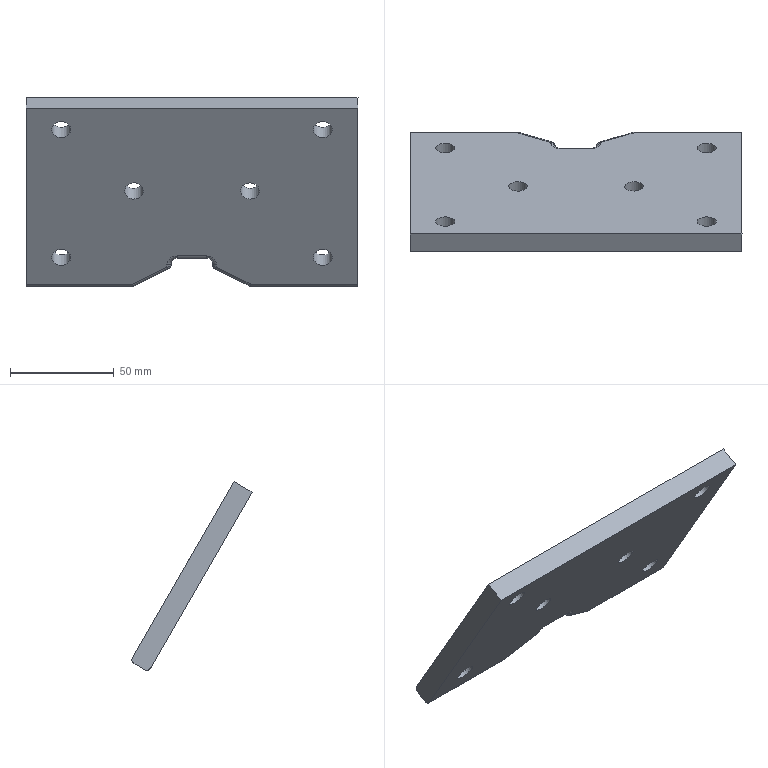Part | NX | features solid 2 | 1 solid | 44 faces | box 160 x 57.93 x 90.87 mm | volume 150907 mm3 | cylinder 23 | plane 12 | torus 4 | sphere 4 | spline 1 | commonest cylinder face diameters 4 x16 9.007 x5 6 x2
STEP:
#1=CARTESIAN_POINT('',(-87.023,177.196,80.17));
#2=VERTEX_POINT('',#1);
#3=CARTESIAN_POINT('',(-87.023,174.944,84.07));
#4=DIRECTION('',(-0.000000832,-0.866,-0.5));
#5=DIRECTION('',(0.,0.5,-0.866));
#6=AXIS2_PLACEMENT_3D('',#3,#4,#5);
#7=CIRCLE('',#6,4.503);
#8=EDGE_CURVE('',#2,#2,#7,.T.);
#9=ORIENTED_EDGE('',*,*,#8,.T.);
#10=EDGE_LOOP('',(#9));
#11=FACE_BOUND('',#10,.T.);
#12=CARTESIAN_POINT('',(-213.023,177.196,80.17));
#13=VERTEX_POINT('',#12);
#14=CARTESIAN_POINT('',(-213.023,174.944,84.07));
#15=DIRECTION('',(-0.000000832,-0.866,-0.5));
#16=DIRECTION('',(0.,0.5,-0.866));
#17=AXIS2_PLACEMENT_3D('',#14,#15,#16);
#18=CIRCLE('',#17,4.503);
#19=EDGE_CURVE('',#13,#13,#18,.T.);
#20=ORIENTED_EDGE('',*,*,#19,.T.);
#21=EDGE_LOOP('',(#20));
#22=FACE_BOUND('',#21,.T.);
#23=CARTESIAN_POINT('',(-213.023,212.697,18.683));
#24=VERTEX_POINT('',#23);
#25=CARTESIAN_POINT('',(-213.023,210.445,22.583));
#26=DIRECTION('',(-0.000000832,-0.866,-0.5));
#27=DIRECTION('',(0.,0.5,-0.866));
#28=AXIS2_PLACEMENT_3D('',#25,#26,#27);
#29=CIRCLE('',#28,4.503);
#30=EDGE_CURVE('',#24,#24,#29,.T.);
#31=ORIENTED_EDGE('',*,*,#30,.T.);
#32=EDGE_LOOP('',(#31));
#33=FACE_BOUND('',#32,.T.);
#34=CARTESIAN_POINT('',(-87.023,212.697,18.683));
#35=VERTEX_POINT('',#34);
#36=CARTESIAN_POINT('',(-87.023,210.445,22.583));
#37=DIRECTION('',(-0.000000832,-0.866,-0.5));
#38=DIRECTION('',(0.,0.5,-0.866));
#39=AXIS2_PLACEMENT_3D('',#36,#37,#38);
#40=CIRCLE('',#39,4.503);
#41=EDGE_CURVE('',#35,#35,#40,.T.);
#42=ORIENTED_EDGE('',*,*,#41,.T.);
#43=EDGE_LOOP('',(#42));
#44=FACE_BOUND('',#43,.T.);
#45=CARTESIAN_POINT('',(-178.024,194.161,50.787));
#46=VERTEX_POINT('',#45);
#47=CARTESIAN_POINT('',(-181.555,193.673,51.632));
#48=CARTESIAN_POINT('',(-178.024,194.405,50.365));
#49=CARTESIAN_POINT('',(-174.496,193.673,51.631));
#50=CARTESIAN_POINT('',(-173.034,191.909,54.688));
#51=CARTESIAN_POINT('',(-174.495,190.144,57.744));
#52=CARTESIAN_POINT('',(-178.023,189.412,59.011));
#53=CARTESIAN_POINT('',(-181.553,190.143,57.745));
#54=CARTESIAN_POINT('',(-183.015,191.908,54.689));
#55=CARTESIAN_POINT('',(-181.555,193.673,51.632));
#56=CARTESIAN_POINT('',(-178.024,194.405,50.365));
#57=CARTESIAN_POINT('',(-174.496,193.673,51.631));
#58=B_SPLINE_CURVE_WITH_KNOTS('',3,(#47,#48,#49,#50,#51,#52,#53,#54,#55,#56,#57),.UNSPECIFIED.,.T.,.F.,(1,1,1,1,1,1,1,1,1,1,1,1,1,1,1),(-0.0106,-0.007066,-0.003533,0.,0.003533,0.007066,0.0106,0.01413,0.01767,0.0212,0.02473,0.02826,0.0318,0.03533,0.03886),.UNSPECIFIED.);
#59=EDGE_CURVE('',#46,#46,#58,.T.);
#60=ORIENTED_EDGE('',*,*,#59,.T.);
#61=EDGE_LOOP('',(#60));
#62=FACE_BOUND('',#61,.T.);
#63=CARTESIAN_POINT('',(-70.023,168.944,94.462));
#64=VERTEX_POINT('',#63);
#65=CARTESIAN_POINT('',(-70.023,217.945,9.593));
#66=VERTEX_POINT('',#65);
#67=CARTESIAN_POINT('',(-70.023,179.194,76.709));
#68=DIRECTION('',(0.000001441,-0.5,0.866));
#69=VECTOR('',#68,1000.);
#70=LINE('',#67,#69);
#71=EDGE_CURVE('',#64,#66,#70,.F.);
#72=ORIENTED_EDGE('',*,*,#71,.T.);
#73=CARTESIAN_POINT('',(-121.568,217.945,9.593));
#74=VERTEX_POINT('',#73);
#75=CARTESIAN_POINT('',(-122.104,217.945,9.593));
#76=DIRECTION('',(1.,0.,-0.000001665));
#77=VECTOR('',#76,1000.);
#78=LINE('',#75,#77);
#79=EDGE_CURVE('',#66,#74,#78,.F.);
#80=ORIENTED_EDGE('',*,*,#79,.T.);
#81=CARTESIAN_POINT('',(-138.099,213.173,17.858));
#82=VERTEX_POINT('',#81);
#83=CARTESIAN_POINT('',(-139.099,212.884,18.358));
#84=DIRECTION('',(-0.866,-0.25,0.433));
#85=VECTOR('',#84,1000.);
#86=LINE('',#83,#85);
#87=EDGE_CURVE('',#74,#82,#86,.T.);
#88=ORIENTED_EDGE('',*,*,#87,.T.);
#89=CARTESIAN_POINT('',(-138.099,212.596,18.858));
#90=VERTEX_POINT('',#89);
#91=CARTESIAN_POINT('',(-138.099,212.596,18.858));
#92=DIRECTION('',(-0.000001442,0.5,-0.866));
#93=VECTOR('',#92,1000.);
#94=LINE('',#91,#93);
#95=EDGE_CURVE('',#82,#90,#94,.F.);
#96=ORIENTED_EDGE('',*,*,#95,.T.);
#97=CARTESIAN_POINT('',(-143.099,210.095,23.188));
#98=VERTEX_POINT('',#97);
#99=CARTESIAN_POINT('',(-143.099,212.596,18.858));
#100=DIRECTION('',(-0.000000832,-0.866,-0.5));
#101=DIRECTION('',(0.,-0.5,0.866));
#102=AXIS2_PLACEMENT_3D('',#99,#100,#101);
#103=CIRCLE('',#102,5.);
#104=EDGE_CURVE('',#90,#98,#103,.T.);
#105=ORIENTED_EDGE('',*,*,#104,.T.);
#106=CARTESIAN_POINT('',(-157.099,210.095,23.188));
#107=VERTEX_POINT('',#106);
#108=CARTESIAN_POINT('',(-157.099,210.095,23.188));
#109=DIRECTION('',(1.,0.,-0.000001665));
#110=VECTOR('',#109,1000.);
#111=LINE('',#108,#110);
#112=EDGE_CURVE('',#98,#107,#111,.F.);
#113=ORIENTED_EDGE('',*,*,#112,.T.);
#114=CARTESIAN_POINT('',(-162.099,212.596,18.858));
#115=VERTEX_POINT('',#114);
#116=CARTESIAN_POINT('',(-157.099,212.596,18.858));
#117=DIRECTION('',(-0.000000832,-0.866,-0.5));
#118=DIRECTION('',(0.,-0.5,0.866));
#119=AXIS2_PLACEMENT_3D('',#116,#117,#118);
#120=CIRCLE('',#119,5.);
#121=EDGE_CURVE('',#107,#115,#120,.T.);
#122=ORIENTED_EDGE('',*,*,#121,.T.);
#123=CARTESIAN_POINT('',(-162.099,213.173,17.858));
#124=VERTEX_POINT('',#123);
#125=CARTESIAN_POINT('',(-162.099,213.75,16.858));
#126=DIRECTION('',(-0.000001441,0.5,-0.866));
#127=VECTOR('',#126,1000.);
#128=LINE('',#125,#127);
#129=EDGE_CURVE('',#115,#124,#128,.T.);
#130=ORIENTED_EDGE('',*,*,#129,.T.);
#131=CARTESIAN_POINT('',(-178.629,217.945,9.593));
#132=VERTEX_POINT('',#131);
#133=CARTESIAN_POINT('',(-179.094,218.079,9.361));
#134=DIRECTION('',(0.866,-0.25,0.433));
#135=VECTOR('',#134,1000.);
#136=LINE('',#133,#135);
#137=EDGE_CURVE('',#124,#132,#136,.F.);
#138=ORIENTED_EDGE('',*,*,#137,.T.);
#139=CARTESIAN_POINT('',(-230.023,217.945,9.593));
#140=VERTEX_POINT('',#139);
#141=CARTESIAN_POINT('',(-230.023,217.945,9.593));
#142=DIRECTION('',(1.,0.,-0.000001665));
#143=VECTOR('',#142,1000.);
#144=LINE('',#141,#143);
#145=EDGE_CURVE('',#132,#140,#144,.F.);
#146=ORIENTED_EDGE('',*,*,#145,.T.);
#147=CARTESIAN_POINT('',(-230.023,168.944,94.463));
#148=VERTEX_POINT('',#147);
#149=CARTESIAN_POINT('',(-230.023,193.925,51.195));
#150=DIRECTION('',(-0.000001441,0.5,-0.866));
#151=VECTOR('',#150,1000.);
#152=LINE('',#149,#151);
#153=EDGE_CURVE('',#148,#140,#152,.T.);
#154=ORIENTED_EDGE('',*,*,#153,.F.);
#155=CARTESIAN_POINT('',(-150.099,168.944,94.463));
#156=DIRECTION('',(-1.,0.,0.000001665));
#157=VECTOR('',#156,1000.);
#158=LINE('',#155,#157);
#159=EDGE_CURVE('',#64,#148,#158,.T.);
#160=ORIENTED_EDGE('',*,*,#159,.F.);
#161=EDGE_LOOP('',(#72,#80,#88,#96,#105,#113,#122,#130,#138,#146,#154,#160));
#162=FACE_BOUND('',#161,.T.);
#163=CARTESIAN_POINT('',(-122.026,194.167,50.777));
#164=VERTEX_POINT('',#163);
#165=CARTESIAN_POINT('',(-122.024,191.914,54.678));
#166=DIRECTION('',(-0.000000832,-0.866,-0.5));
#167=DIRECTION('',(-0.0003265,0.5,-0.866));
#168=AXIS2_PLACEMENT_3D('',#165,#166,#167);
#169=ELLIPSE('',#168,4.504,4.503);
#170=EDGE_CURVE('',#164,#164,#169,.F.);
#171=ORIENTED_EDGE('',*,*,#170,.F.);
#172=EDGE_LOOP('',(#171));
#173=FACE_BOUND('',#172,.T.);
#174=CARTESIAN_POINT('',(-150.099,193.925,51.195));
#175=DIRECTION('',(-0.000000832,-0.866,-0.5));
#176=DIRECTION('',(0.000001441,-0.5,0.866));
#177=AXIS2_PLACEMENT_3D('',#174,#175,#176);
#178=PLANE('',#177);
#179=ADVANCED_FACE('',(#11,#22,#33,#44,#62,#162,#173),#178,.F.);
#180=CARTESIAN_POINT('',(-87.023,168.536,75.17));
#181=VERTEX_POINT('',#180);
#182=CARTESIAN_POINT('',(-87.023,166.284,79.07));
#183=DIRECTION('',(-0.000000832,-0.866,-0.5));
#184=DIRECTION('',(0.,0.5,-0.866));
#185=AXIS2_PLACEMENT_3D('',#182,#183,#184);
#186=CIRCLE('',#185,4.503);
#187=EDGE_CURVE('',#181,#181,#186,.T.);
#188=ORIENTED_EDGE('',*,*,#187,.F.);
#189=EDGE_LOOP('',(#188));
#190=FACE_BOUND('',#189,.T.);
#191=CARTESIAN_POINT('',(-213.023,168.536,75.17));
#192=VERTEX_POINT('',#191);
#193=CARTESIAN_POINT('',(-213.023,166.284,79.07));
#194=DIRECTION('',(-0.000000832,-0.866,-0.5));
#195=DIRECTION('',(0.,0.5,-0.866));
#196=AXIS2_PLACEMENT_3D('',#193,#194,#195);
#197=CIRCLE('',#196,4.503);
#198=EDGE_CURVE('',#192,#192,#197,.T.);
#199=ORIENTED_EDGE('',*,*,#198,.F.);
#200=EDGE_LOOP('',(#199));
#201=FACE_BOUND('',#200,.T.);
#202=CARTESIAN_POINT('',(-213.023,204.036,13.683));
#203=VERTEX_POINT('',#202);
#204=CARTESIAN_POINT('',(-213.023,201.785,17.583));
#205=DIRECTION('',(-0.000000832,-0.866,-0.5));
#206=DIRECTION('',(0.,0.5,-0.866));
#207=AXIS2_PLACEMENT_3D('',#204,#205,#206);
#208=CIRCLE('',#207,4.503);
#209=EDGE_CURVE('',#203,#203,#208,.T.);
#210=ORIENTED_EDGE('',*,*,#209,.F.);
#211=EDGE_LOOP('',(#210));
#212=FACE_BOUND('',#211,.T.);
#213=CARTESIAN_POINT('',(-87.023,204.036,13.683));
#214=VERTEX_POINT('',#213);
#215=CARTESIAN_POINT('',(-87.023,201.785,17.583));
#216=DIRECTION('',(-0.000000832,-0.866,-0.5));
#217=DIRECTION('',(0.,0.5,-0.866));
#218=AXIS2_PLACEMENT_3D('',#215,#216,#217);
#219=CIRCLE('',#218,4.503);
#220=EDGE_CURVE('',#214,#214,#219,.T.);
#221=ORIENTED_EDGE('',*,*,#220,.F.);
#222=EDGE_LOOP('',(#221));
#223=FACE_BOUND('',#222,.T.);
#224=CARTESIAN_POINT('',(-178.024,185.601,45.614));
#225=VERTEX_POINT('',#224);
#226=CARTESIAN_POINT('',(-181.555,185.112,46.459));
#227=CARTESIAN_POINT('',(-178.024,185.844,45.191));
#228=CARTESIAN_POINT('',(-174.496,185.113,46.458));
#229=CARTESIAN_POINT('',(-173.034,183.348,49.514));
#230=CARTESIAN_POINT('',(-174.495,181.584,52.571));
#231=CARTESIAN_POINT('',(-178.023,180.852,53.838));
#232=CARTESIAN_POINT('',(-181.553,181.583,52.572));
#233=CARTESIAN_POINT('',(-183.015,183.348,49.516));
#234=CARTESIAN_POINT('',(-181.555,185.112,46.459));
#235=CARTESIAN_POINT('',(-178.024,185.844,45.191));
#236=CARTESIAN_POINT('',(-174.496,185.113,46.458));
#237=B_SPLINE_CURVE_WITH_KNOTS('',3,(#226,#227,#228,#229,#230,#231,#232,#233,#234,#235,#236),.UNSPECIFIED.,.T.,.F.,(1,1,1,1,1,1,1,1,1,1,1,1,1,1,1),(-0.0106,-0.007066,-0.003533,0.,0.003533,0.007066,0.0106,0.01413,0.01767,0.0212,0.02473,0.02826,0.0318,0.03533,0.03886),.UNSPECIFIED.);
#238=EDGE_CURVE('',#225,#225,#237,.T.);
#239=ORIENTED_EDGE('',*,*,#238,.F.);
#240=EDGE_LOOP('',(#239));
#241=FACE_BOUND('',#240,.T.);
#242=CARTESIAN_POINT('',(-138.099,204.513,12.858));
#243=VERTEX_POINT('',#242);
#244=CARTESIAN_POINT('',(-121.568,209.285,4.593));
#245=VERTEX_POINT('',#244);
#246=CARTESIAN_POINT('',(-163.767,197.103,25.692));
#247=DIRECTION('',(0.866,0.25,-0.433));
#248=VECTOR('',#247,1000.);
#249=LINE('',#246,#248);
#250=EDGE_CURVE('',#243,#245,#249,.T.);
#251=ORIENTED_EDGE('',*,*,#250,.T.);
#252=CARTESIAN_POINT('',(-70.023,209.285,4.593));
#253=VERTEX_POINT('',#252);
#254=CARTESIAN_POINT('',(-150.099,209.285,4.593));
#255=DIRECTION('',(1.,0.,-0.000001665));
#256=VECTOR('',#255,1000.);
#257=LINE('',#254,#256);
#258=EDGE_CURVE('',#245,#253,#257,.T.);
#259=ORIENTED_EDGE('',*,*,#258,.T.);
#260=CARTESIAN_POINT('',(-70.023,160.283,89.462));
#261=VERTEX_POINT('',#260);
#262=CARTESIAN_POINT('',(-70.023,170.534,71.709));
#263=DIRECTION('',(0.000001441,-0.5,0.866));
#264=VECTOR('',#263,1000.);
#265=LINE('',#262,#264);
#266=EDGE_CURVE('',#261,#253,#265,.F.);
#267=ORIENTED_EDGE('',*,*,#266,.F.);
#268=CARTESIAN_POINT('',(-230.023,160.283,89.463));
#269=VERTEX_POINT('',#268);
#270=CARTESIAN_POINT('',(-150.099,160.283,89.462));
#271=DIRECTION('',(-1.,0.,0.000001665));
#272=VECTOR('',#271,1000.);
#273=LINE('',#270,#272);
#274=EDGE_CURVE('',#261,#269,#273,.T.);
#275=ORIENTED_EDGE('',*,*,#274,.T.);
#276=CARTESIAN_POINT('',(-230.023,209.285,4.593));
#277=VERTEX_POINT('',#276);
#278=CARTESIAN_POINT('',(-230.023,185.265,46.195));
#279=DIRECTION('',(-0.000001441,0.5,-0.866));
#280=VECTOR('',#279,1000.);
#281=LINE('',#278,#280);
#282=EDGE_CURVE('',#269,#277,#281,.T.);
#283=ORIENTED_EDGE('',*,*,#282,.T.);
#284=CARTESIAN_POINT('',(-178.629,209.285,4.593));
#285=VERTEX_POINT('',#284);
#286=CARTESIAN_POINT('',(-150.099,209.285,4.593));
#287=DIRECTION('',(1.,0.,-0.000001665));
#288=VECTOR('',#287,1000.);
#289=LINE('',#286,#288);
#290=EDGE_CURVE('',#277,#285,#289,.T.);
#291=ORIENTED_EDGE('',*,*,#290,.T.);
#292=CARTESIAN_POINT('',(-162.099,204.513,12.858));
#293=VERTEX_POINT('',#292);
#294=CARTESIAN_POINT('',(-136.43,197.103,25.692));
#295=DIRECTION('',(-0.866,0.25,-0.433));
#296=VECTOR('',#295,1000.);
#297=LINE('',#294,#296);
#298=EDGE_CURVE('',#285,#293,#297,.F.);
#299=ORIENTED_EDGE('',*,*,#298,.T.);
#300=CARTESIAN_POINT('',(-162.099,203.935,13.858));
#301=VERTEX_POINT('',#300);
#302=CARTESIAN_POINT('',(-162.099,185.265,46.195));
#303=DIRECTION('',(-0.000001441,0.5,-0.866));
#304=VECTOR('',#303,1000.);
#305=LINE('',#302,#304);
#306=EDGE_CURVE('',#293,#301,#305,.F.);
#307=ORIENTED_EDGE('',*,*,#306,.T.);
#308=CARTESIAN_POINT('',(-157.099,201.435,18.188));
#309=VERTEX_POINT('',#308);
#310=CARTESIAN_POINT('',(-157.099,203.935,13.858));
#311=DIRECTION('',(-0.000000832,-0.866,-0.5));
#312=DIRECTION('',(0.,-0.5,0.866));
#313=AXIS2_PLACEMENT_3D('',#310,#311,#312);
#314=CIRCLE('',#313,5.);
#315=EDGE_CURVE('',#301,#309,#314,.F.);
#316=ORIENTED_EDGE('',*,*,#315,.T.);
#317=CARTESIAN_POINT('',(-143.099,201.435,18.188));
#318=VERTEX_POINT('',#317);
#319=CARTESIAN_POINT('',(-150.099,201.435,18.188));
#320=DIRECTION('',(-1.,0.,0.000001665));
#321=VECTOR('',#320,1000.);
#322=LINE('',#319,#321);
#323=EDGE_CURVE('',#309,#318,#322,.F.);
#324=ORIENTED_EDGE('',*,*,#323,.T.);
#325=CARTESIAN_POINT('',(-138.099,203.935,13.858));
#326=VERTEX_POINT('',#325);
#327=CARTESIAN_POINT('',(-143.099,203.935,13.858));
#328=DIRECTION('',(-0.000000832,-0.866,-0.5));
#329=DIRECTION('',(0.,-0.5,0.866));
#330=AXIS2_PLACEMENT_3D('',#327,#328,#329);
#331=CIRCLE('',#330,5.);
#332=EDGE_CURVE('',#318,#326,#331,.F.);
#333=ORIENTED_EDGE('',*,*,#332,.T.);
#334=CARTESIAN_POINT('',(-138.099,185.265,46.195));
#335=DIRECTION('',(-0.000001442,0.5,-0.866));
#336=VECTOR('',#335,1000.);
#337=LINE('',#334,#336);
#338=EDGE_CURVE('',#326,#243,#337,.T.);
#339=ORIENTED_EDGE('',*,*,#338,.T.);
#340=EDGE_LOOP('',(#251,#259,#267,#275,#283,#291,#299,#307,#316,#324,#333,#339));
#341=FACE_BOUND('',#340,.T.);
#342=CARTESIAN_POINT('',(-122.026,185.607,45.603));
#343=VERTEX_POINT('',#342);
#344=CARTESIAN_POINT('',(-122.024,183.354,49.504));
#345=DIRECTION('',(-0.000000832,-0.866,-0.5));
#346=DIRECTION('',(-0.0003265,0.5,-0.866));
#347=AXIS2_PLACEMENT_3D('',#344,#345,#346);
#348=ELLIPSE('',#347,4.504,4.503);
#349=EDGE_CURVE('',#343,#343,#348,.F.);
#350=ORIENTED_EDGE('',*,*,#349,.T.);
#351=EDGE_LOOP('',(#350));
#352=FACE_BOUND('',#351,.T.);
#353=CARTESIAN_POINT('',(-150.099,185.265,46.195));
#354=DIRECTION('',(-0.000000832,-0.866,-0.5));
#355=DIRECTION('',(0.000001441,-0.5,0.866));
#356=AXIS2_PLACEMENT_3D('',#353,#354,#355);
#357=PLANE('',#356);
#358=ADVANCED_FACE('',(#190,#201,#212,#223,#241,#341,#352),#357,.T.);
#359=CARTESIAN_POINT('',(-230.023,212.017,3.861));
#360=VERTEX_POINT('',#359);
#361=CARTESIAN_POINT('',(-230.023,217.213,6.861));
#362=VERTEX_POINT('',#361);
#363=CARTESIAN_POINT('',(-230.023,183.993,-12.319));
#364=DIRECTION('',(-0.000000832,-0.866,-0.5));
#365=VECTOR('',#364,1000.);
#366=LINE('',#363,#365);
#367=EDGE_CURVE('',#360,#362,#366,.F.);
#368=ORIENTED_EDGE('',*,*,#367,.T.);
#369=CARTESIAN_POINT('',(-178.094,217.213,6.861));
#370=VERTEX_POINT('',#369);
#371=CARTESIAN_POINT('',(-178.094,217.213,6.861));
#372=DIRECTION('',(-1.,0.,0.000001665));
#373=VECTOR('',#372,1000.);
#374=LINE('',#371,#373);
#375=EDGE_CURVE('',#362,#370,#374,.F.);
#376=ORIENTED_EDGE('',*,*,#375,.T.);
#377=CARTESIAN_POINT('',(-178.094,212.017,3.861));
#378=VERTEX_POINT('',#377);
#379=CARTESIAN_POINT('',(-178.094,183.993,-12.319));
#380=DIRECTION('',(0.000001182,0.866,0.5));
#381=VECTOR('',#380,1000.);
#382=LINE('',#379,#381);
#383=EDGE_CURVE('',#370,#378,#382,.F.);
#384=ORIENTED_EDGE('',*,*,#383,.T.);
#385=CARTESIAN_POINT('',(-150.023,212.017,3.861));
#386=DIRECTION('',(-1.,0.,0.000001665));
#387=VECTOR('',#386,1000.);
#388=LINE('',#385,#387);
#389=EDGE_CURVE('',#378,#360,#388,.T.);
#390=ORIENTED_EDGE('',*,*,#389,.T.);
#391=EDGE_LOOP('',(#368,#376,#384,#390));
#392=FACE_BOUND('',#391,.T.);
#393=CARTESIAN_POINT('',(-150.023,183.993,-12.319));
#394=DIRECTION('',(0.000001441,-0.5,0.866));
#395=DIRECTION('',(0.000000832,0.866,0.5));
#396=AXIS2_PLACEMENT_3D('',#393,#394,#395);
#397=PLANE('',#396);
#398=ADVANCED_FACE('',(#392),#397,.F.);
#399=CARTESIAN_POINT('',(-122.104,217.213,6.861));
#400=VERTEX_POINT('',#399);
#401=CARTESIAN_POINT('',(-122.104,212.017,3.861));
#402=VERTEX_POINT('',#401);
#403=CARTESIAN_POINT('',(-122.104,556.807,202.933));
#404=DIRECTION('',(0.000000483,0.866,0.5));
#405=VECTOR('',#404,1000.);
#406=LINE('',#403,#405);
#407=EDGE_CURVE('',#400,#402,#406,.F.);
#408=ORIENTED_EDGE('',*,*,#407,.F.);
#409=CARTESIAN_POINT('',(-70.023,217.213,6.861));
#410=VERTEX_POINT('',#409);
#411=CARTESIAN_POINT('',(-70.023,217.213,6.861));
#412=DIRECTION('',(-1.,0.,0.000001665));
#413=VECTOR('',#412,1000.);
#414=LINE('',#411,#413);
#415=EDGE_CURVE('',#400,#410,#414,.F.);
#416=ORIENTED_EDGE('',*,*,#415,.T.);
#417=CARTESIAN_POINT('',(-70.023,212.017,3.861));
#418=VERTEX_POINT('',#417);
#419=CARTESIAN_POINT('',(-70.023,210.285,2.861));
#420=DIRECTION('',(0.000000832,0.866,0.5));
#421=VECTOR('',#420,1000.);
#422=LINE('',#419,#421);
#423=EDGE_CURVE('',#418,#410,#422,.T.);
#424=ORIENTED_EDGE('',*,*,#423,.F.);
#425=CARTESIAN_POINT('',(-150.023,212.017,3.861));
#426=DIRECTION('',(-1.,0.,0.000001665));
#427=VECTOR('',#426,1000.);
#428=LINE('',#425,#427);
#429=EDGE_CURVE('',#418,#402,#428,.T.);
#430=ORIENTED_EDGE('',*,*,#429,.T.);
#431=EDGE_LOOP('',(#408,#416,#424,#430));
#432=FACE_BOUND('',#431,.T.);
#433=CARTESIAN_POINT('',(-150.023,183.993,-12.319));
#434=DIRECTION('',(0.000001441,-0.5,0.866));
#435=DIRECTION('',(0.000000832,0.866,0.5));
#436=AXIS2_PLACEMENT_3D('',#433,#434,#435);
#437=PLANE('',#436);
#438=ADVANCED_FACE('',(#432),#437,.F.);
#439=CARTESIAN_POINT('',(-230.023,160.283,89.463));
#440=DIRECTION('',(0.000000832,0.866,0.5));
#441=VECTOR('',#440,1000.);
#442=LINE('',#439,#441);
#443=EDGE_CURVE('',#269,#148,#442,.T.);
#444=ORIENTED_EDGE('',*,*,#443,.F.);
#445=ORIENTED_EDGE('',*,*,#274,.F.);
#446=CARTESIAN_POINT('',(-70.023,133.992,74.282));
#447=DIRECTION('',(-0.000000832,-0.866,-0.5));
#448=VECTOR('',#447,1000.);
#449=LINE('',#446,#448);
#450=EDGE_CURVE('',#261,#64,#449,.F.);
#451=ORIENTED_EDGE('',*,*,#450,.T.);
#452=ORIENTED_EDGE('',*,*,#159,.T.);
#453=EDGE_LOOP('',(#444,#445,#451,#452));
#454=FACE_BOUND('',#453,.T.);
#455=CARTESIAN_POINT('',(-150.023,133.992,74.283));
#456=DIRECTION('',(0.000001441,-0.5,0.866));
#457=DIRECTION('',(0.000000832,0.866,0.5));
#458=AXIS2_PLACEMENT_3D('',#455,#456,#457);
#459=PLANE('',#458);
#460=ADVANCED_FACE('',(#454),#459,.T.);
#461=ORIENTED_EDGE('',*,*,#423,.T.);
#462=CARTESIAN_POINT('',(-70.023,216.213,8.593));
#463=DIRECTION('',(-1.,0.,0.000001665));
#464=DIRECTION('',(-0.000001665,0.,-1.));
#465=AXIS2_PLACEMENT_3D('',#462,#463,#464);
#466=CIRCLE('',#465,2.);
#467=EDGE_CURVE('',#410,#66,#466,.F.);
#468=ORIENTED_EDGE('',*,*,#467,.T.);
#469=ORIENTED_EDGE('',*,*,#71,.F.);
#470=ORIENTED_EDGE('',*,*,#450,.F.);
#471=ORIENTED_EDGE('',*,*,#266,.T.);
#472=CARTESIAN_POINT('',(-70.023,211.017,5.593));
#473=DIRECTION('',(-1.,0.,0.000001665));
#474=DIRECTION('',(-0.000001665,0.,-1.));
#475=AXIS2_PLACEMENT_3D('',#472,#473,#474);
#476=CIRCLE('',#475,2.);
#477=EDGE_CURVE('',#253,#418,#476,.F.);
#478=ORIENTED_EDGE('',*,*,#477,.T.);
#479=EDGE_LOOP('',(#461,#468,#469,#470,#471,#478));
#480=FACE_BOUND('',#479,.T.);
#481=CARTESIAN_POINT('',(-70.023,170.534,71.709));
#482=DIRECTION('',(-1.,0.,0.000001665));
#483=DIRECTION('',(-0.000001441,0.5,-0.866));
#484=AXIS2_PLACEMENT_3D('',#481,#482,#483);
#485=PLANE('',#484);
#486=ADVANCED_FACE('',(#480),#485,.F.);
#487=ORIENTED_EDGE('',*,*,#153,.T.);
#488=CARTESIAN_POINT('',(-230.023,216.213,8.593));
#489=DIRECTION('',(-1.,0.,0.000001665));
#490=DIRECTION('',(-0.000001665,0.,-1.));
#491=AXIS2_PLACEMENT_3D('',#488,#489,#490);
#492=CIRCLE('',#491,2.);
#493=EDGE_CURVE('',#140,#362,#492,.T.);
#494=ORIENTED_EDGE('',*,*,#493,.T.);
#495=ORIENTED_EDGE('',*,*,#367,.F.);
#496=CARTESIAN_POINT('',(-230.023,211.017,5.593));
#497=DIRECTION('',(-1.,0.,0.000001665));
#498=DIRECTION('',(-0.000001665,0.,-1.));
#499=AXIS2_PLACEMENT_3D('',#496,#497,#498);
#500=CIRCLE('',#499,2.);
#501=EDGE_CURVE('',#360,#277,#500,.T.);
#502=ORIENTED_EDGE('',*,*,#501,.T.);
#503=ORIENTED_EDGE('',*,*,#282,.F.);
#504=ORIENTED_EDGE('',*,*,#443,.T.);
#505=EDGE_LOOP('',(#487,#494,#495,#502,#503,#504));
#506=FACE_BOUND('',#505,.T.);
#507=CARTESIAN_POINT('',(-230.023,185.265,46.195));
#508=DIRECTION('',(-1.,0.,0.000001665));
#509=DIRECTION('',(-0.000001441,0.5,-0.866));
#510=AXIS2_PLACEMENT_3D('',#507,#508,#509);
#511=PLANE('',#510);
#512=ADVANCED_FACE('',(#506),#511,.T.);
#513=CARTESIAN_POINT('',(-161.099,212.307,15.358));
#514=VERTEX_POINT('',#513);
#515=CARTESIAN_POINT('',(-160.099,212.018,15.858));
#516=DIRECTION('',(0.866,-0.25,0.433));
#517=VECTOR('',#516,1000.);
#518=LINE('',#515,#517);
#519=EDGE_CURVE('',#370,#514,#518,.T.);
#520=ORIENTED_EDGE('',*,*,#519,.T.);
#521=CARTESIAN_POINT('',(-161.099,207.111,12.358));
#522=VERTEX_POINT('',#521);
#523=CARTESIAN_POINT('',(-161.098,551.901,211.43));
#524=DIRECTION('',(-0.000000832,-0.866,-0.5));
#525=VECTOR('',#524,1000.);
#526=LINE('',#523,#525);
#527=EDGE_CURVE('',#514,#522,#526,.T.);
#528=ORIENTED_EDGE('',*,*,#527,.T.);
#529=CARTESIAN_POINT('',(-177.58,211.869,4.118));
#530=DIRECTION('',(-0.866,0.25,-0.433));
#531=VECTOR('',#530,1000.);
#532=LINE('',#529,#531);
#533=EDGE_CURVE('',#522,#378,#532,.T.);
#534=ORIENTED_EDGE('',*,*,#533,.T.);
#535=ORIENTED_EDGE('',*,*,#383,.F.);
#536=EDGE_LOOP('',(#520,#528,#534,#535));
#537=FACE_BOUND('',#536,.T.);
#538=CARTESIAN_POINT('',(-177.579,556.659,203.19));
#539=DIRECTION('',(0.5,0.433,-0.75));
#540=DIRECTION('',(0.832,0.,0.5547));
#541=AXIS2_PLACEMENT_3D('',#538,#539,#540);
#542=PLANE('',#541);
#543=ADVANCED_FACE('',(#537),#542,.T.);
#544=CARTESIAN_POINT('',(-160.099,205.667,14.858));
#545=VERTEX_POINT('',#544);
#546=CARTESIAN_POINT('',(-160.099,206.245,13.858));
#547=VERTEX_POINT('',#546);
#548=CARTESIAN_POINT('',(-160.099,207.688,11.358));
#549=DIRECTION('',(-0.000001441,0.5,-0.866));
#550=VECTOR('',#549,1000.);
#551=LINE('',#548,#550);
#552=EDGE_CURVE('',#545,#547,#551,.T.);
#553=ORIENTED_EDGE('',*,*,#552,.T.);
#554=CARTESIAN_POINT('',(-160.099,211.441,16.858));
#555=VERTEX_POINT('',#554);
#556=CARTESIAN_POINT('',(-160.098,551.035,212.93));
#557=DIRECTION('',(-0.000000832,-0.866,-0.5));
#558=VECTOR('',#557,1000.);
#559=LINE('',#556,#558);
#560=EDGE_CURVE('',#547,#555,#559,.F.);
#561=ORIENTED_EDGE('',*,*,#560,.T.);
#562=CARTESIAN_POINT('',(-160.099,210.864,17.858));
#563=VERTEX_POINT('',#562);
#564=CARTESIAN_POINT('',(-160.099,210.864,17.858));
#565=DIRECTION('',(-0.000001441,0.5,-0.866));
#566=VECTOR('',#565,1000.);
#567=LINE('',#564,#566);
#568=EDGE_CURVE('',#555,#563,#567,.F.);
#569=ORIENTED_EDGE('',*,*,#568,.T.);
#570=CARTESIAN_POINT('',(-160.099,203.935,13.858));
#571=DIRECTION('',(-0.000000832,-0.866,-0.5));
#572=VECTOR('',#571,1000.);
#573=LINE('',#570,#572);
#574=EDGE_CURVE('',#563,#545,#573,.T.);
#575=ORIENTED_EDGE('',*,*,#574,.T.);
#576=EDGE_LOOP('',(#553,#561,#569,#575));
#577=FACE_BOUND('',#576,.T.);
#578=CARTESIAN_POINT('',(-160.098,552.479,210.43));
#579=DIRECTION('',(1.,0.,-0.000001664));
#580=DIRECTION('',(0.000001664,0.,1.));
#581=AXIS2_PLACEMENT_3D('',#578,#579,#580);
#582=PLANE('',#581);
#583=ADVANCED_FACE('',(#577),#582,.T.);
#584=CARTESIAN_POINT('',(-157.099,204.167,17.456));
#585=VERTEX_POINT('',#584);
#586=CARTESIAN_POINT('',(-157.099,209.363,20.456));
#587=VERTEX_POINT('',#586);
#588=CARTESIAN_POINT('',(-157.099,211.095,21.456));
#589=DIRECTION('',(-0.000000832,-0.866,-0.5));
#590=VECTOR('',#589,1000.);
#591=LINE('',#588,#590);
#592=EDGE_CURVE('',#585,#587,#591,.F.);
#593=ORIENTED_EDGE('',*,*,#592,.T.);
#594=CARTESIAN_POINT('',(-143.099,209.363,20.456));
#595=VERTEX_POINT('',#594);
#596=CARTESIAN_POINT('',(-143.099,209.363,20.456));
#597=DIRECTION('',(1.,0.,-0.000001665));
#598=VECTOR('',#597,1000.);
#599=LINE('',#596,#598);
#600=EDGE_CURVE('',#587,#595,#599,.T.);
#601=ORIENTED_EDGE('',*,*,#600,.T.);
#602=CARTESIAN_POINT('',(-143.099,204.167,17.456));
#603=VERTEX_POINT('',#602);
#604=CARTESIAN_POINT('',(-143.099,202.435,16.456));
#605=DIRECTION('',(-0.000000832,-0.866,-0.5));
#606=VECTOR('',#605,1000.);
#607=LINE('',#604,#606);
#608=EDGE_CURVE('',#595,#603,#607,.T.);
#609=ORIENTED_EDGE('',*,*,#608,.T.);
#610=CARTESIAN_POINT('',(-157.099,204.167,17.456));
#611=DIRECTION('',(-1.,0.,0.000001665));
#612=VECTOR('',#611,1000.);
#613=LINE('',#610,#612);
#614=EDGE_CURVE('',#603,#585,#613,.T.);
#615=ORIENTED_EDGE('',*,*,#614,.T.);
#616=EDGE_LOOP('',(#593,#601,#609,#615));
#617=FACE_BOUND('',#616,.T.);
#618=CARTESIAN_POINT('',(-157.098,548.958,216.528));
#619=DIRECTION('',(-0.000001441,0.5,-0.866));
#620=DIRECTION('',(0.,-0.866,-0.5));
#621=AXIS2_PLACEMENT_3D('',#618,#619,#620);
#622=PLANE('',#621);
#623=ADVANCED_FACE('',(#617),#622,.T.);
#624=CARTESIAN_POINT('',(-140.099,210.864,17.858));
#625=VERTEX_POINT('',#624);
#626=CARTESIAN_POINT('',(-140.099,211.441,16.858));
#627=VERTEX_POINT('',#626);
#628=CARTESIAN_POINT('',(-140.099,212.018,15.858));
#629=DIRECTION('',(-0.000001442,0.5,-0.866));
#630=VECTOR('',#629,1000.);
#631=LINE('',#628,#630);
#632=EDGE_CURVE('',#625,#627,#631,.T.);
#633=ORIENTED_EDGE('',*,*,#632,.T.);
#634=CARTESIAN_POINT('',(-140.099,206.245,13.858));
#635=VERTEX_POINT('',#634);
#636=CARTESIAN_POINT('',(-140.098,551.035,212.93));
#637=DIRECTION('',(-0.000000832,-0.866,-0.5));
#638=VECTOR('',#637,1000.);
#639=LINE('',#636,#638);
#640=EDGE_CURVE('',#627,#635,#639,.T.);
#641=ORIENTED_EDGE('',*,*,#640,.T.);
#642=CARTESIAN_POINT('',(-140.099,205.667,14.858));
#643=VERTEX_POINT('',#642);
#644=CARTESIAN_POINT('',(-140.099,205.667,14.858));
#645=DIRECTION('',(-0.000001442,0.5,-0.866));
#646=VECTOR('',#645,1000.);
#647=LINE('',#644,#646);
#648=EDGE_CURVE('',#635,#643,#647,.F.);
#649=ORIENTED_EDGE('',*,*,#648,.T.);
#650=CARTESIAN_POINT('',(-140.099,212.596,18.858));
#651=DIRECTION('',(-0.000000832,-0.866,-0.5));
#652=VECTOR('',#651,1000.);
#653=LINE('',#650,#652);
#654=EDGE_CURVE('',#643,#625,#653,.F.);
#655=ORIENTED_EDGE('',*,*,#654,.T.);
#656=EDGE_LOOP('',(#633,#641,#649,#655));
#657=FACE_BOUND('',#656,.T.);
#658=CARTESIAN_POINT('',(-140.098,550.458,213.93));
#659=DIRECTION('',(-1.,0.,0.000001665));
#660=DIRECTION('',(-0.000001665,0.,-1.));
#661=AXIS2_PLACEMENT_3D('',#658,#659,#660);
#662=PLANE('',#661);
#663=ADVANCED_FACE('',(#657),#662,.T.);
#664=CARTESIAN_POINT('',(-139.099,207.111,12.358));
#665=VERTEX_POINT('',#664);
#666=CARTESIAN_POINT('',(-141.599,206.389,13.608));
#667=DIRECTION('',(0.866,0.25,-0.433));
#668=VECTOR('',#667,1000.);
#669=LINE('',#666,#668);
#670=EDGE_CURVE('',#402,#665,#669,.F.);
#671=ORIENTED_EDGE('',*,*,#670,.T.);
#672=CARTESIAN_POINT('',(-139.099,212.307,15.358));
#673=VERTEX_POINT('',#672);
#674=CARTESIAN_POINT('',(-139.098,551.901,211.43));
#675=DIRECTION('',(-0.000000832,-0.866,-0.5));
#676=VECTOR('',#675,1000.);
#677=LINE('',#674,#676);
#678=EDGE_CURVE('',#665,#673,#677,.F.);
#679=ORIENTED_EDGE('',*,*,#678,.T.);
#680=CARTESIAN_POINT('',(-122.104,217.213,6.861));
#681=DIRECTION('',(-0.866,-0.25,0.433));
#682=VECTOR('',#681,1000.);
#683=LINE('',#680,#682);
#684=EDGE_CURVE('',#673,#400,#683,.F.);
#685=ORIENTED_EDGE('',*,*,#684,.T.);
#686=ORIENTED_EDGE('',*,*,#407,.T.);
#687=EDGE_LOOP('',(#671,#679,#685,#686));
#688=FACE_BOUND('',#687,.T.);
#689=CARTESIAN_POINT('',(-141.598,551.18,212.68));
#690=DIRECTION('',(-0.5,0.433,-0.75));
#691=DIRECTION('',(0.832,0.,-0.5547));
#692=AXIS2_PLACEMENT_3D('',#689,#690,#691);
#693=PLANE('',#692);
#694=ADVANCED_FACE('',(#688),#693,.T.);
#695=ORIENTED_EDGE('',*,*,#608,.F.);
#696=CARTESIAN_POINT('',(-143.099,210.864,17.858));
#697=DIRECTION('',(-0.000000832,-0.866,-0.5));
#698=DIRECTION('',(0.,-0.5,0.866));
#699=AXIS2_PLACEMENT_3D('',#696,#697,#698);
#700=CIRCLE('',#699,3.);
#701=EDGE_CURVE('',#595,#625,#700,.F.);
#702=ORIENTED_EDGE('',*,*,#701,.T.);
#703=ORIENTED_EDGE('',*,*,#654,.F.);
#704=CARTESIAN_POINT('',(-143.099,205.667,14.858));
#705=DIRECTION('',(-0.000000832,-0.866,-0.5));
#706=DIRECTION('',(0.,-0.5,0.866));
#707=AXIS2_PLACEMENT_3D('',#704,#705,#706);
#708=CIRCLE('',#707,3.);
#709=EDGE_CURVE('',#643,#603,#708,.T.);
#710=ORIENTED_EDGE('',*,*,#709,.T.);
#711=EDGE_LOOP('',(#695,#702,#703,#710));
#712=FACE_BOUND('',#711,.T.);
#713=CARTESIAN_POINT('',(-143.098,550.458,213.93));
#714=DIRECTION('',(0.000000832,0.866,0.5));
#715=DIRECTION('',(0.,0.5,-0.866));
#716=AXIS2_PLACEMENT_3D('',#713,#714,#715);
#717=CYLINDRICAL_SURFACE('',#716,3.);
#718=ADVANCED_FACE('',(#712),#717,.F.);
#719=ORIENTED_EDGE('',*,*,#574,.F.);
#720=CARTESIAN_POINT('',(-157.099,210.864,17.858));
#721=DIRECTION('',(-0.000000832,-0.866,-0.5));
#722=DIRECTION('',(0.,-0.5,0.866));
#723=AXIS2_PLACEMENT_3D('',#720,#721,#722);
#724=CIRCLE('',#723,3.);
#725=EDGE_CURVE('',#563,#587,#724,.F.);
#726=ORIENTED_EDGE('',*,*,#725,.T.);
#727=ORIENTED_EDGE('',*,*,#592,.F.);
#728=CARTESIAN_POINT('',(-157.099,205.667,14.858));
#729=DIRECTION('',(-0.000000832,-0.866,-0.5));
#730=DIRECTION('',(0.,-0.5,0.866));
#731=AXIS2_PLACEMENT_3D('',#728,#729,#730);
#732=CIRCLE('',#731,3.);
#733=EDGE_CURVE('',#585,#545,#732,.T.);
#734=ORIENTED_EDGE('',*,*,#733,.T.);
#735=EDGE_LOOP('',(#719,#726,#727,#734));
#736=FACE_BOUND('',#735,.T.);
#737=CARTESIAN_POINT('',(-157.098,550.458,213.93));
#738=DIRECTION('',(0.000000832,0.866,0.5));
#739=DIRECTION('',(0.,0.5,-0.866));
#740=AXIS2_PLACEMENT_3D('',#737,#738,#739);
#741=CYLINDRICAL_SURFACE('',#740,3.);
#742=ADVANCED_FACE('',(#736),#741,.F.);
#743=ORIENTED_EDGE('',*,*,#493,.F.);
#744=ORIENTED_EDGE('',*,*,#145,.F.);
#745=CARTESIAN_POINT('',(-178.629,216.213,8.593));
#746=DIRECTION('',(-0.9659,0.1294,-0.2241));
#747=DIRECTION('',(-0.2588,-0.483,0.8365));
#748=AXIS2_PLACEMENT_3D('',#745,#746,#747);
#749=ELLIPSE('',#748,2.071,2.);
#750=EDGE_CURVE('',#370,#132,#749,.F.);
#751=ORIENTED_EDGE('',*,*,#750,.F.);
#752=ORIENTED_EDGE('',*,*,#375,.F.);
#753=EDGE_LOOP('',(#743,#744,#751,#752));
#754=FACE_BOUND('',#753,.T.);
#755=CARTESIAN_POINT('',(-150.099,216.213,8.593));
#756=DIRECTION('',(-1.,0.,0.000001665));
#757=DIRECTION('',(-0.000001665,0.,-1.));
#758=AXIS2_PLACEMENT_3D('',#755,#756,#757);
#759=CYLINDRICAL_SURFACE('',#758,2.);
#760=ADVANCED_FACE('',(#754),#759,.T.);
#761=ORIENTED_EDGE('',*,*,#137,.F.);
#762=CARTESIAN_POINT('',(-162.099,211.441,16.858));
#763=DIRECTION('',(-0.866,0.25,-0.433));
#764=DIRECTION('',(0.4472,0.,-0.8944));
#765=AXIS2_PLACEMENT_3D('',#762,#763,#764);
#766=CIRCLE('',#765,2.);
#767=EDGE_CURVE('',#124,#514,#766,.T.);
#768=ORIENTED_EDGE('',*,*,#767,.T.);
#769=ORIENTED_EDGE('',*,*,#519,.F.);
#770=ORIENTED_EDGE('',*,*,#750,.T.);
#771=EDGE_LOOP('',(#761,#768,#769,#770));
#772=FACE_BOUND('',#771,.T.);
#773=CARTESIAN_POINT('',(-178.58,216.199,8.618));
#774=DIRECTION('',(-0.866,0.25,-0.433));
#775=DIRECTION('',(0.4472,0.,-0.8944));
#776=AXIS2_PLACEMENT_3D('',#773,#774,#775);
#777=CYLINDRICAL_SURFACE('',#776,2.);
#778=ADVANCED_FACE('',(#772),#777,.T.);
#779=ORIENTED_EDGE('',*,*,#568,.F.);
#780=CARTESIAN_POINT('',(-162.099,211.441,16.858));
#781=DIRECTION('',(0.000001441,-0.5,0.866));
#782=DIRECTION('',(0.,0.866,0.5));
#783=AXIS2_PLACEMENT_3D('',#780,#781,#782);
#784=CIRCLE('',#783,2.);
#785=EDGE_CURVE('',#555,#124,#784,.T.);
#786=ORIENTED_EDGE('',*,*,#785,.T.);
#787=ORIENTED_EDGE('',*,*,#129,.F.);
#788=CARTESIAN_POINT('',(-162.099,210.864,17.858));
#789=DIRECTION('',(0.000001441,-0.5,0.866));
#790=DIRECTION('',(0.,0.866,0.5));
#791=AXIS2_PLACEMENT_3D('',#788,#789,#790);
#792=CIRCLE('',#791,2.);
#793=EDGE_CURVE('',#563,#115,#792,.T.);
#794=ORIENTED_EDGE('',*,*,#793,.F.);
#795=EDGE_LOOP('',(#779,#786,#787,#794));
#796=FACE_BOUND('',#795,.T.);
#797=CARTESIAN_POINT('',(-162.099,192.193,50.195));
#798=DIRECTION('',(0.000001441,-0.5,0.866));
#799=DIRECTION('',(0.,0.866,0.5));
#800=AXIS2_PLACEMENT_3D('',#797,#798,#799);
#801=CYLINDRICAL_SURFACE('',#800,2.);
#802=ADVANCED_FACE('',(#796),#801,.T.);
#803=ORIENTED_EDGE('',*,*,#793,.T.);
#804=ORIENTED_EDGE('',*,*,#121,.F.);
#805=CARTESIAN_POINT('',(-157.099,208.363,22.188));
#806=DIRECTION('',(1.,0.,-0.000001665));
#807=DIRECTION('',(0.000001665,0.,1.));
#808=AXIS2_PLACEMENT_3D('',#805,#806,#807);
#809=CIRCLE('',#808,2.);
#810=EDGE_CURVE('',#587,#107,#809,.T.);
#811=ORIENTED_EDGE('',*,*,#810,.F.);
#812=ORIENTED_EDGE('',*,*,#725,.F.);
#813=EDGE_LOOP('',(#803,#804,#811,#812));
#814=FACE_BOUND('',#813,.T.);
#815=CARTESIAN_POINT('',(-157.099,210.864,17.858));
#816=DIRECTION('',(-0.000000832,-0.866,-0.5));
#817=DIRECTION('',(0.,-0.5,0.866));
#818=AXIS2_PLACEMENT_3D('',#815,#816,#817);
#819=TOROIDAL_SURFACE('',#818,5.,2.);
#820=ADVANCED_FACE('',(#814),#819,.T.);
#821=ORIENTED_EDGE('',*,*,#810,.T.);
#822=ORIENTED_EDGE('',*,*,#112,.F.);
#823=CARTESIAN_POINT('',(-143.099,208.363,22.188));
#824=DIRECTION('',(1.,0.,-0.000001665));
#825=DIRECTION('',(0.000001665,0.,1.));
#826=AXIS2_PLACEMENT_3D('',#823,#824,#825);
#827=CIRCLE('',#826,2.);
#828=EDGE_CURVE('',#595,#98,#827,.T.);
#829=ORIENTED_EDGE('',*,*,#828,.F.);
#830=ORIENTED_EDGE('',*,*,#600,.F.);
#831=EDGE_LOOP('',(#821,#822,#829,#830));
#832=FACE_BOUND('',#831,.T.);
#833=CARTESIAN_POINT('',(-157.099,208.363,22.188));
#834=DIRECTION('',(-1.,0.,0.000001665));
#835=DIRECTION('',(-0.000001665,0.,-1.));
#836=AXIS2_PLACEMENT_3D('',#833,#834,#835);
#837=CYLINDRICAL_SURFACE('',#836,2.);
#838=ADVANCED_FACE('',(#832),#837,.T.);
#839=ORIENTED_EDGE('',*,*,#467,.F.);
#840=ORIENTED_EDGE('',*,*,#415,.F.);
#841=CARTESIAN_POINT('',(-121.568,216.213,8.593));
#842=DIRECTION('',(0.9659,0.1294,-0.2241));
#843=DIRECTION('',(-0.2588,0.483,-0.8365));
#844=AXIS2_PLACEMENT_3D('',#841,#842,#843);
#845=ELLIPSE('',#844,2.071,2.);
#846=EDGE_CURVE('',#74,#400,#845,.F.);
#847=ORIENTED_EDGE('',*,*,#846,.F.);
#848=ORIENTED_EDGE('',*,*,#79,.F.);
#849=EDGE_LOOP('',(#839,#840,#847,#848));
#850=FACE_BOUND('',#849,.T.);
#851=CARTESIAN_POINT('',(-150.099,216.213,8.593));
#852=DIRECTION('',(-1.,0.,0.000001665));
#853=DIRECTION('',(-0.000001665,0.,-1.));
#854=AXIS2_PLACEMENT_3D('',#851,#852,#853);
#855=CYLINDRICAL_SURFACE('',#854,2.);
#856=ADVANCED_FACE('',(#850),#855,.T.);
#857=ORIENTED_EDGE('',*,*,#828,.T.);
#858=ORIENTED_EDGE('',*,*,#104,.F.);
#859=CARTESIAN_POINT('',(-138.099,210.864,17.858));
#860=DIRECTION('',(-0.000001442,0.5,-0.866));
#861=DIRECTION('',(0.,-0.866,-0.5));
#862=AXIS2_PLACEMENT_3D('',#859,#860,#861);
#863=CIRCLE('',#862,2.);
#864=EDGE_CURVE('',#625,#90,#863,.T.);
#865=ORIENTED_EDGE('',*,*,#864,.F.);
#866=ORIENTED_EDGE('',*,*,#701,.F.);
#867=EDGE_LOOP('',(#857,#858,#865,#866));
#868=FACE_BOUND('',#867,.T.);
#869=CARTESIAN_POINT('',(-143.099,210.864,17.858));
#870=DIRECTION('',(-0.000000832,-0.866,-0.5));
#871=DIRECTION('',(0.,-0.5,0.866));
#872=AXIS2_PLACEMENT_3D('',#869,#870,#871);
#873=TOROIDAL_SURFACE('',#872,5.,2.);
#874=ADVANCED_FACE('',(#868),#873,.T.);
#875=ORIENTED_EDGE('',*,*,#684,.F.);
#876=CARTESIAN_POINT('',(-138.099,211.441,16.858));
#877=DIRECTION('',(0.866,0.25,-0.433));
#878=DIRECTION('',(0.4472,0.,0.8944));
#879=AXIS2_PLACEMENT_3D('',#876,#877,#878);
#880=CIRCLE('',#879,2.);
#881=EDGE_CURVE('',#673,#82,#880,.T.);
#882=ORIENTED_EDGE('',*,*,#881,.T.);
#883=ORIENTED_EDGE('',*,*,#87,.F.);
#884=ORIENTED_EDGE('',*,*,#846,.T.);
#885=EDGE_LOOP('',(#875,#882,#883,#884));
#886=FACE_BOUND('',#885,.T.);
#887=CARTESIAN_POINT('',(-163.767,204.031,29.692));
#888=DIRECTION('',(0.866,0.25,-0.433));
#889=DIRECTION('',(0.4472,0.,0.8944));
#890=AXIS2_PLACEMENT_3D('',#887,#888,#889);
#891=CYLINDRICAL_SURFACE('',#890,2.);
#892=ADVANCED_FACE('',(#886),#891,.T.);
#893=ORIENTED_EDGE('',*,*,#95,.F.);
#894=CARTESIAN_POINT('',(-138.099,211.441,16.858));
#895=DIRECTION('',(0.000001442,-0.5,0.866));
#896=DIRECTION('',(0.,0.866,0.5));
#897=AXIS2_PLACEMENT_3D('',#894,#895,#896);
#898=CIRCLE('',#897,2.);
#899=EDGE_CURVE('',#82,#627,#898,.T.);
#900=ORIENTED_EDGE('',*,*,#899,.T.);
#901=ORIENTED_EDGE('',*,*,#632,.F.);
#902=ORIENTED_EDGE('',*,*,#864,.T.);
#903=EDGE_LOOP('',(#893,#900,#901,#902));
#904=FACE_BOUND('',#903,.T.);
#905=CARTESIAN_POINT('',(-138.099,210.864,17.858));
#906=DIRECTION('',(0.000001442,-0.5,0.866));
#907=DIRECTION('',(0.,0.866,0.5));
#908=AXIS2_PLACEMENT_3D('',#905,#906,#907);
#909=CYLINDRICAL_SURFACE('',#908,2.);
#910=ADVANCED_FACE('',(#904),#909,.T.);
#911=ORIENTED_EDGE('',*,*,#501,.F.);
#912=ORIENTED_EDGE('',*,*,#389,.F.);
#913=CARTESIAN_POINT('',(-178.629,211.017,5.593));
#914=DIRECTION('',(0.9659,-0.1294,0.2241));
#915=DIRECTION('',(0.2588,0.483,-0.8365));
#916=AXIS2_PLACEMENT_3D('',#913,#914,#915);
#917=ELLIPSE('',#916,2.071,2.);
#918=EDGE_CURVE('',#285,#378,#917,.T.);
#919=ORIENTED_EDGE('',*,*,#918,.F.);
#920=ORIENTED_EDGE('',*,*,#290,.F.);
#921=EDGE_LOOP('',(#911,#912,#919,#920));
#922=FACE_BOUND('',#921,.T.);
#923=CARTESIAN_POINT('',(-150.023,211.017,5.593));
#924=DIRECTION('',(1.,0.,-0.000001665));
#925=DIRECTION('',(0.000001665,0.,1.));
#926=AXIS2_PLACEMENT_3D('',#923,#924,#925);
#927=CYLINDRICAL_SURFACE('',#926,2.);
#928=ADVANCED_FACE('',(#922),#927,.T.);
#929=ORIENTED_EDGE('',*,*,#533,.F.);
#930=CARTESIAN_POINT('',(-162.099,206.245,13.858));
#931=DIRECTION('',(-0.866,0.25,-0.433));
#932=DIRECTION('',(0.4472,0.,-0.8944));
#933=AXIS2_PLACEMENT_3D('',#930,#931,#932);
#934=CIRCLE('',#933,2.);
#935=EDGE_CURVE('',#522,#293,#934,.T.);
#936=ORIENTED_EDGE('',*,*,#935,.T.);
#937=ORIENTED_EDGE('',*,*,#298,.F.);
#938=ORIENTED_EDGE('',*,*,#918,.T.);
#939=EDGE_LOOP('',(#929,#936,#937,#938));
#940=FACE_BOUND('',#939,.T.);
#941=CARTESIAN_POINT('',(-178.58,211.002,5.618));
#942=DIRECTION('',(-0.866,0.25,-0.433));
#943=DIRECTION('',(0.4472,0.,-0.8944));
#944=AXIS2_PLACEMENT_3D('',#941,#942,#943);
#945=CYLINDRICAL_SURFACE('',#944,2.);
#946=ADVANCED_FACE('',(#940),#945,.T.);
#947=ORIENTED_EDGE('',*,*,#306,.F.);
#948=CARTESIAN_POINT('',(-162.099,206.245,13.858));
#949=DIRECTION('',(-0.000001441,0.5,-0.866));
#950=DIRECTION('',(0.,-0.866,-0.5));
#951=AXIS2_PLACEMENT_3D('',#948,#949,#950);
#952=CIRCLE('',#951,2.);
#953=EDGE_CURVE('',#293,#547,#952,.F.);
#954=ORIENTED_EDGE('',*,*,#953,.T.);
#955=ORIENTED_EDGE('',*,*,#552,.F.);
#956=CARTESIAN_POINT('',(-162.099,205.667,14.858));
#957=DIRECTION('',(0.000001441,-0.5,0.866));
#958=DIRECTION('',(0.,0.866,0.5));
#959=AXIS2_PLACEMENT_3D('',#956,#957,#958);
#960=CIRCLE('',#959,2.);
#961=EDGE_CURVE('',#301,#545,#960,.T.);
#962=ORIENTED_EDGE('',*,*,#961,.F.);
#963=EDGE_LOOP('',(#947,#954,#955,#962));
#964=FACE_BOUND('',#963,.T.);
#965=CARTESIAN_POINT('',(-162.099,207.688,11.358));
#966=DIRECTION('',(-0.000001441,0.5,-0.866));
#967=DIRECTION('',(0.,-0.866,-0.5));
#968=AXIS2_PLACEMENT_3D('',#965,#966,#967);
#969=CYLINDRICAL_SURFACE('',#968,2.);
#970=ADVANCED_FACE('',(#964),#969,.T.);
#971=ORIENTED_EDGE('',*,*,#961,.T.);
#972=ORIENTED_EDGE('',*,*,#733,.F.);
#973=CARTESIAN_POINT('',(-157.099,203.167,19.188));
#974=DIRECTION('',(1.,0.,-0.000001665));
#975=DIRECTION('',(0.000001665,0.,1.));
#976=AXIS2_PLACEMENT_3D('',#973,#974,#975);
#977=CIRCLE('',#976,2.);
#978=EDGE_CURVE('',#309,#585,#977,.T.);
#979=ORIENTED_EDGE('',*,*,#978,.F.);
#980=ORIENTED_EDGE('',*,*,#315,.F.);
#981=EDGE_LOOP('',(#971,#972,#979,#980));
#982=FACE_BOUND('',#981,.T.);
#983=CARTESIAN_POINT('',(-157.099,205.667,14.858));
#984=DIRECTION('',(-0.000000832,-0.866,-0.5));
#985=DIRECTION('',(0.,-0.5,0.866));
#986=AXIS2_PLACEMENT_3D('',#983,#984,#985);
#987=TOROIDAL_SURFACE('',#986,5.,2.);
#988=ADVANCED_FACE('',(#982),#987,.T.);
#989=ORIENTED_EDGE('',*,*,#978,.T.);
#990=ORIENTED_EDGE('',*,*,#614,.F.);
#991=CARTESIAN_POINT('',(-143.099,203.167,19.188));
#992=DIRECTION('',(1.,0.,-0.000001665));
#993=DIRECTION('',(0.000001665,0.,1.));
#994=AXIS2_PLACEMENT_3D('',#991,#992,#993);
#995=CIRCLE('',#994,2.);
#996=EDGE_CURVE('',#318,#603,#995,.T.);
#997=ORIENTED_EDGE('',*,*,#996,.F.);
#998=ORIENTED_EDGE('',*,*,#323,.F.);
#999=EDGE_LOOP('',(#989,#990,#997,#998));
#1000=FACE_BOUND('',#999,.T.);
#1001=CARTESIAN_POINT('',(-157.099,203.167,19.188));
#1002=DIRECTION('',(-1.,0.,0.000001665));
#1003=DIRECTION('',(-0.000001665,0.,-1.));
#1004=AXIS2_PLACEMENT_3D('',#1001,#1002,#1003);
#1005=CYLINDRICAL_SURFACE('',#1004,2.);
#1006=ADVANCED_FACE('',(#1000),#1005,.T.);
#1007=ORIENTED_EDGE('',*,*,#996,.T.);
#1008=ORIENTED_EDGE('',*,*,#709,.F.);
#1009=CARTESIAN_POINT('',(-138.099,205.667,14.858));
#1010=DIRECTION('',(-0.000001442,0.5,-0.866));
#1011=DIRECTION('',(0.,-0.866,-0.5));
#1012=AXIS2_PLACEMENT_3D('',#1009,#1010,#1011);
#1013=CIRCLE('',#1012,2.);
#1014=EDGE_CURVE('',#326,#643,#1013,.T.);
#1015=ORIENTED_EDGE('',*,*,#1014,.F.);
#1016=ORIENTED_EDGE('',*,*,#332,.F.);
#1017=EDGE_LOOP('',(#1007,#1008,#1015,#1016));
#1018=FACE_BOUND('',#1017,.T.);
#1019=CARTESIAN_POINT('',(-143.099,205.667,14.858));
#1020=DIRECTION('',(-0.000000832,-0.866,-0.5));
#1021=DIRECTION('',(0.,-0.5,0.866));
#1022=AXIS2_PLACEMENT_3D('',#1019,#1020,#1021);
#1023=TOROIDAL_SURFACE('',#1022,5.,2.);
#1024=ADVANCED_FACE('',(#1018),#1023,.T.);
#1025=ORIENTED_EDGE('',*,*,#648,.F.);
#1026=CARTESIAN_POINT('',(-138.099,206.245,13.858));
#1027=DIRECTION('',(-0.000001442,0.5,-0.866));
#1028=DIRECTION('',(0.,-0.866,-0.5));
#1029=AXIS2_PLACEMENT_3D('',#1026,#1027,#1028);
#1030=CIRCLE('',#1029,2.);
#1031=EDGE_CURVE('',#635,#243,#1030,.F.);
#1032=ORIENTED_EDGE('',*,*,#1031,.T.);
#1033=ORIENTED_EDGE('',*,*,#338,.F.);
#1034=ORIENTED_EDGE('',*,*,#1014,.T.);
#1035=EDGE_LOOP('',(#1025,#1032,#1033,#1034));
#1036=FACE_BOUND('',#1035,.T.);
#1037=CARTESIAN_POINT('',(-138.099,186.997,47.195));
#1038=DIRECTION('',(-0.000001442,0.5,-0.866));
#1039=DIRECTION('',(0.,-0.866,-0.5));
#1040=AXIS2_PLACEMENT_3D('',#1037,#1038,#1039);
#1041=CYLINDRICAL_SURFACE('',#1040,2.);
#1042=ADVANCED_FACE('',(#1036),#1041,.T.);
#1043=ORIENTED_EDGE('',*,*,#250,.F.);
#1044=CARTESIAN_POINT('',(-138.099,206.245,13.858));
#1045=DIRECTION('',(0.866,0.25,-0.433));
#1046=DIRECTION('',(0.4472,0.,0.8944));
#1047=AXIS2_PLACEMENT_3D('',#1044,#1045,#1046);
#1048=CIRCLE('',#1047,2.);
#1049=EDGE_CURVE('',#243,#665,#1048,.T.);
#1050=ORIENTED_EDGE('',*,*,#1049,.T.);
#1051=ORIENTED_EDGE('',*,*,#670,.F.);
#1052=CARTESIAN_POINT('',(-121.568,211.017,5.593));
#1053=DIRECTION('',(0.9659,0.1294,-0.2241));
#1054=DIRECTION('',(-0.2588,0.483,-0.8365));
#1055=AXIS2_PLACEMENT_3D('',#1052,#1053,#1054);
#1056=ELLIPSE('',#1055,2.071,2.);
#1057=EDGE_CURVE('',#245,#402,#1056,.T.);
#1058=ORIENTED_EDGE('',*,*,#1057,.F.);
#1059=EDGE_LOOP('',(#1043,#1050,#1051,#1058));
#1060=FACE_BOUND('',#1059,.T.);
#1061=CARTESIAN_POINT('',(-163.767,198.835,26.692));
#1062=DIRECTION('',(0.866,0.25,-0.433));
#1063=DIRECTION('',(0.4472,0.,0.8944));
#1064=AXIS2_PLACEMENT_3D('',#1061,#1062,#1063);
#1065=CYLINDRICAL_SURFACE('',#1064,2.);
#1066=ADVANCED_FACE('',(#1060),#1065,.T.);
#1067=ORIENTED_EDGE('',*,*,#477,.F.);
#1068=ORIENTED_EDGE('',*,*,#258,.F.);
#1069=ORIENTED_EDGE('',*,*,#1057,.T.);
#1070=ORIENTED_EDGE('',*,*,#429,.F.);
#1071=EDGE_LOOP('',(#1067,#1068,#1069,#1070));
#1072=FACE_BOUND('',#1071,.T.);
#1073=CARTESIAN_POINT('',(-150.023,211.017,5.593));
#1074=DIRECTION('',(1.,0.,-0.000001665));
#1075=DIRECTION('',(0.000001665,0.,1.));
#1076=AXIS2_PLACEMENT_3D('',#1073,#1074,#1075);
#1077=CYLINDRICAL_SURFACE('',#1076,2.);
#1078=ADVANCED_FACE('',(#1072),#1077,.T.);
#1079=ORIENTED_EDGE('',*,*,#1049,.F.);
#1080=ORIENTED_EDGE('',*,*,#1031,.F.);
#1081=CARTESIAN_POINT('',(-138.099,206.245,13.858));
#1082=DIRECTION('',(0.000000832,0.866,0.5));
#1083=DIRECTION('',(0.,0.5,-0.866));
#1084=AXIS2_PLACEMENT_3D('',#1081,#1082,#1083);
#1085=CIRCLE('',#1084,2.);
#1086=EDGE_CURVE('',#665,#635,#1085,.T.);
#1087=ORIENTED_EDGE('',*,*,#1086,.F.);
#1088=EDGE_LOOP('',(#1079,#1080,#1087));
#1089=FACE_BOUND('',#1088,.T.);
#1090=CARTESIAN_POINT('',(-138.099,206.245,13.858));
#1091=DIRECTION('',(0.,0.,1.));
#1092=DIRECTION('',(-1.,0.,0.));
#1093=AXIS2_PLACEMENT_3D('',#1090,#1091,#1092);
#1094=SPHERICAL_SURFACE('',#1093,2.);
#1095=ADVANCED_FACE('',(#1089),#1094,.T.);
#1096=ORIENTED_EDGE('',*,*,#1086,.T.);
#1097=ORIENTED_EDGE('',*,*,#640,.F.);
#1098=CARTESIAN_POINT('',(-138.099,211.441,16.858));
#1099=DIRECTION('',(0.000000832,0.866,0.5));
#1100=DIRECTION('',(0.,0.5,-0.866));
#1101=AXIS2_PLACEMENT_3D('',#1098,#1099,#1100);
#1102=CIRCLE('',#1101,2.);
#1103=EDGE_CURVE('',#673,#627,#1102,.T.);
#1104=ORIENTED_EDGE('',*,*,#1103,.F.);
#1105=ORIENTED_EDGE('',*,*,#678,.F.);
#1106=EDGE_LOOP('',(#1096,#1097,#1104,#1105));
#1107=FACE_BOUND('',#1106,.T.);
#1108=CARTESIAN_POINT('',(-138.098,551.035,212.93));
#1109=DIRECTION('',(-0.000000832,-0.866,-0.5));
#1110=DIRECTION('',(0.,-0.5,0.866));
#1111=AXIS2_PLACEMENT_3D('',#1108,#1109,#1110);
#1112=CYLINDRICAL_SURFACE('',#1111,2.);
#1113=ADVANCED_FACE('',(#1107),#1112,.T.);
#1114=ORIENTED_EDGE('',*,*,#899,.F.);
#1115=ORIENTED_EDGE('',*,*,#881,.F.);
#1116=ORIENTED_EDGE('',*,*,#1103,.T.);
#1117=EDGE_LOOP('',(#1114,#1115,#1116));
#1118=FACE_BOUND('',#1117,.T.);
#1119=CARTESIAN_POINT('',(-138.099,211.441,16.858));
#1120=DIRECTION('',(0.,0.,1.));
#1121=DIRECTION('',(-1.,0.,0.));
#1122=AXIS2_PLACEMENT_3D('',#1119,#1120,#1121);
#1123=SPHERICAL_SURFACE('',#1122,2.);
#1124=ADVANCED_FACE('',(#1118),#1123,.T.);
#1125=ORIENTED_EDGE('',*,*,#953,.F.);
#1126=ORIENTED_EDGE('',*,*,#935,.F.);
#1127=CARTESIAN_POINT('',(-162.099,206.245,13.858));
#1128=DIRECTION('',(0.000000832,0.866,0.5));
#1129=DIRECTION('',(0.,0.5,-0.866));
#1130=AXIS2_PLACEMENT_3D('',#1127,#1128,#1129);
#1131=CIRCLE('',#1130,2.);
#1132=EDGE_CURVE('',#547,#522,#1131,.T.);
#1133=ORIENTED_EDGE('',*,*,#1132,.F.);
#1134=EDGE_LOOP('',(#1125,#1126,#1133));
#1135=FACE_BOUND('',#1134,.T.);
#1136=CARTESIAN_POINT('',(-162.099,206.245,13.858));
#1137=DIRECTION('',(0.,0.,1.));
#1138=DIRECTION('',(-1.,0.,0.));
#1139=AXIS2_PLACEMENT_3D('',#1136,#1137,#1138);
#1140=SPHERICAL_SURFACE('',#1139,2.);
#1141=ADVANCED_FACE('',(#1135),#1140,.T.);
#1142=ORIENTED_EDGE('',*,*,#1132,.T.);
#1143=ORIENTED_EDGE('',*,*,#527,.F.);
#1144=CARTESIAN_POINT('',(-162.099,211.441,16.858));
#1145=DIRECTION('',(0.000000832,0.866,0.5));
#1146=DIRECTION('',(0.,0.5,-0.866));
#1147=AXIS2_PLACEMENT_3D('',#1144,#1145,#1146);
#1148=CIRCLE('',#1147,2.);
#1149=EDGE_CURVE('',#555,#514,#1148,.T.);
#1150=ORIENTED_EDGE('',*,*,#1149,.F.);
#1151=ORIENTED_EDGE('',*,*,#560,.F.);
#1152=EDGE_LOOP('',(#1142,#1143,#1150,#1151));
#1153=FACE_BOUND('',#1152,.T.);
#1154=CARTESIAN_POINT('',(-162.098,551.035,212.93));
#1155=DIRECTION('',(-0.000000832,-0.866,-0.5));
#1156=DIRECTION('',(0.,-0.5,0.866));
#1157=AXIS2_PLACEMENT_3D('',#1154,#1155,#1156);
#1158=CYLINDRICAL_SURFACE('',#1157,2.);
#1159=ADVANCED_FACE('',(#1153),#1158,.T.);
#1160=ORIENTED_EDGE('',*,*,#1149,.T.);
#1161=ORIENTED_EDGE('',*,*,#767,.F.);
#1162=ORIENTED_EDGE('',*,*,#785,.F.);
#1163=EDGE_LOOP('',(#1160,#1161,#1162));
#1164=FACE_BOUND('',#1163,.T.);
#1165=CARTESIAN_POINT('',(-162.099,211.441,16.858));
#1166=DIRECTION('',(0.,0.,1.));
#1167=DIRECTION('',(-1.,0.,0.));
#1168=AXIS2_PLACEMENT_3D('',#1165,#1166,#1167);
#1169=SPHERICAL_SURFACE('',#1168,2.);
#1170=ADVANCED_FACE('',(#1164),#1169,.T.);
#1171=ORIENTED_EDGE('',*,*,#349,.F.);
#1172=EDGE_LOOP('',(#1171));
#1173=FACE_BOUND('',#1172,.T.);
#1174=ORIENTED_EDGE('',*,*,#170,.T.);
#1175=EDGE_LOOP('',(#1174));
#1176=FACE_BOUND('',#1175,.T.);
#1177=CARTESIAN_POINT('',(-122.016,1159.615,639.528));
#1178=DIRECTION('',(-0.000007365,-0.8558,-0.5172));
#1179=DIRECTION('',(0.,0.5172,-0.8558));
#1180=AXIS2_PLACEMENT_3D('',#1177,#1178,#1179);
#1181=CYLINDRICAL_SURFACE('',#1180,4.503);
#1182=ADVANCED_FACE('',(#1173,#1176),#1181,.F.);
#1183=ORIENTED_EDGE('',*,*,#238,.T.);
#1184=EDGE_LOOP('',(#1183));
#1185=FACE_BOUND('',#1184,.T.);
#1186=ORIENTED_EDGE('',*,*,#59,.F.);
#1187=EDGE_LOOP('',(#1186));
#1188=FACE_BOUND('',#1187,.T.);
#1189=CARTESIAN_POINT('',(-181.553,193.863,51.746));
#1190=CARTESIAN_POINT('',(-181.553,185.044,46.416));
#1191=CARTESIAN_POINT('',(-178.024,194.619,50.495));
#1192=CARTESIAN_POINT('',(-178.024,185.8,45.165));
#1193=CARTESIAN_POINT('',(-174.495,193.863,51.746));
#1194=CARTESIAN_POINT('',(-174.495,185.044,46.416));
#1195=CARTESIAN_POINT('',(-173.034,192.038,54.766));
#1196=CARTESIAN_POINT('',(-173.034,183.219,49.436));
#1197=CARTESIAN_POINT('',(-174.495,190.213,57.787));
#1198=CARTESIAN_POINT('',(-174.495,181.393,52.457));
#1199=CARTESIAN_POINT('',(-178.024,189.456,59.038));
#1200=CARTESIAN_POINT('',(-178.024,180.637,53.708));
#1201=CARTESIAN_POINT('',(-181.553,190.213,57.787));
#1202=CARTESIAN_POINT('',(-181.553,181.394,52.457));
#1203=CARTESIAN_POINT('',(-183.015,192.038,54.766));
#1204=CARTESIAN_POINT('',(-183.015,183.219,49.436));
#1205=CARTESIAN_POINT('',(-181.553,193.863,51.746));
#1206=CARTESIAN_POINT('',(-181.553,185.044,46.416));
#1207=CARTESIAN_POINT('',(-178.024,194.619,50.495));
#1208=CARTESIAN_POINT('',(-178.024,185.8,45.165));
#1209=CARTESIAN_POINT('',(-174.495,193.863,51.746));
#1210=CARTESIAN_POINT('',(-174.495,185.044,46.416));
#1211=B_SPLINE_SURFACE_WITH_KNOTS('',3,1,((#1189,#1190),(#1191,#1192),(#1193,#1194),(#1195,#1196),(#1197,#1198),(#1199,#1200),(#1201,#1202),(#1203,#1204),(#1205,#1206),(#1207,#1208),(#1209,#1210)),.SURF_OF_LINEAR_EXTRUSION.,.T.,.F.,.F.,(1,1,1,1,1,1,1,1,1,1,1,1,1,1,1),(2,2),(-2.356,-1.571,-0.7854,0.,0.7854,1.571,2.356,3.142,3.927,4.712,5.498,6.283,7.069,7.854,8.639),(0.,1.),.UNSPECIFIED.);
#1212=ADVANCED_FACE('',(#1185,#1188),#1211,.F.);
#1213=ORIENTED_EDGE('',*,*,#220,.T.);
#1214=EDGE_LOOP('',(#1213));
#1215=FACE_BOUND('',#1214,.T.);
#1216=ORIENTED_EDGE('',*,*,#41,.F.);
#1217=EDGE_LOOP('',(#1216));
#1218=FACE_BOUND('',#1217,.T.);
#1219=CARTESIAN_POINT('',(-87.022,1220.221,605.599));
#1220=DIRECTION('',(-0.000000832,-0.866,-0.5));
#1221=DIRECTION('',(0.,0.5,-0.866));
#1222=AXIS2_PLACEMENT_3D('',#1219,#1220,#1221);
#1223=CYLINDRICAL_SURFACE('',#1222,4.503);
#1224=ADVANCED_FACE('',(#1215,#1218),#1223,.F.);
#1225=ORIENTED_EDGE('',*,*,#209,.T.);
#1226=EDGE_LOOP('',(#1225));
#1227=FACE_BOUND('',#1226,.T.);
#1228=ORIENTED_EDGE('',*,*,#30,.F.);
#1229=EDGE_LOOP('',(#1228));
#1230=FACE_BOUND('',#1229,.T.);
#1231=CARTESIAN_POINT('',(-213.022,1220.221,605.6));
#1232=DIRECTION('',(-0.000000832,-0.866,-0.5));
#1233=DIRECTION('',(0.,0.5,-0.866));
#1234=AXIS2_PLACEMENT_3D('',#1231,#1232,#1233);
#1235=CYLINDRICAL_SURFACE('',#1234,4.503);
#1236=ADVANCED_FACE('',(#1227,#1230),#1235,.F.);
#1237=ORIENTED_EDGE('',*,*,#198,.T.);
#1238=EDGE_LOOP('',(#1237));
#1239=FACE_BOUND('',#1238,.T.);
#1240=ORIENTED_EDGE('',*,*,#19,.F.);
#1241=EDGE_LOOP('',(#1240));
#1242=FACE_BOUND('',#1241,.T.);
#1243=CARTESIAN_POINT('',(-213.022,1184.72,667.087));
#1244=DIRECTION('',(-0.000000832,-0.866,-0.5));
#1245=DIRECTION('',(0.,0.5,-0.866));
#1246=AXIS2_PLACEMENT_3D('',#1243,#1244,#1245);
#1247=CYLINDRICAL_SURFACE('',#1246,4.503);
#1248=ADVANCED_FACE('',(#1239,#1242),#1247,.F.);
#1249=ORIENTED_EDGE('',*,*,#187,.T.);
#1250=EDGE_LOOP('',(#1249));
#1251=FACE_BOUND('',#1250,.T.);
#1252=ORIENTED_EDGE('',*,*,#8,.F.);
#1253=EDGE_LOOP('',(#1252));
#1254=FACE_BOUND('',#1253,.T.);
#1255=CARTESIAN_POINT('',(-87.022,1184.72,667.087));
#1256=DIRECTION('',(-0.000000832,-0.866,-0.5));
#1257=DIRECTION('',(0.,0.5,-0.866));
#1258=AXIS2_PLACEMENT_3D('',#1255,#1256,#1257);
#1259=CYLINDRICAL_SURFACE('',#1258,4.503);
#1260=ADVANCED_FACE('',(#1251,#1254),#1259,.F.);
#1261=CLOSED_SHELL('',(#179,#358,#398,#438,#460,#486,#512,#543,#583,#623,#663,#694,#718,#742,#760,#778,#802,#820,#838,#856,#874,#892,#910,#928,#946,#970,#988,#1006,#1024,#1042,#1066,#1078,#1095,#1113,#1124,#1141,#1159,#1170,#1182,#1212,#1224,#1236,#1248,#1260));
#1262=MANIFOLD_SOLID_BREP('',#1261);
#1263=(LENGTH_UNIT()NAMED_UNIT(*)SI_UNIT(.MILLI.,.METRE.));
#1264=UNCERTAINTY_MEASURE_WITH_UNIT(LENGTH_MEASURE(0.0508),#1263,'','');
#1265=(NAMED_UNIT(*)PLANE_ANGLE_UNIT()SI_UNIT($,.RADIAN.));
#1266=(NAMED_UNIT(*)SI_UNIT($,.STERADIAN.)SOLID_ANGLE_UNIT());
#1267=(GEOMETRIC_REPRESENTATION_CONTEXT(3)GLOBAL_UNCERTAINTY_ASSIGNED_CONTEXT((#1264))GLOBAL_UNIT_ASSIGNED_CONTEXT((#1263,#1265,#1266))REPRESENTATION_CONTEXT('',''));
#1268=ADVANCED_BREP_SHAPE_REPRESENTATION('',(#1262),#1267);